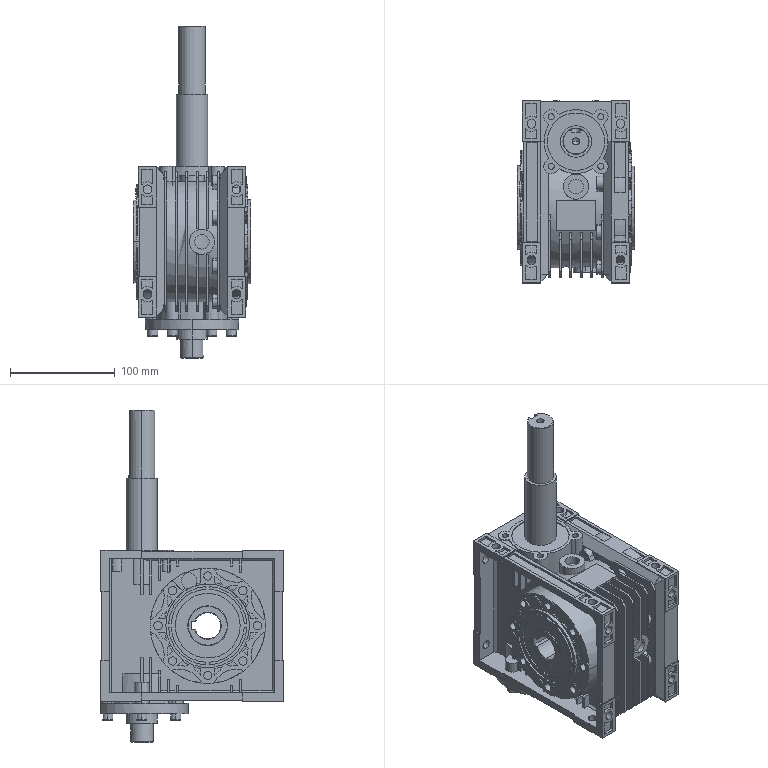Part | SolidWorks | features BaseBody 1 | 1 solid | 1734 faces | box 112 x 174 x 317 mm | volume 1817597 mm3 | plane 991 | cylinder 692 | spline 28 | cone 23 | commonest cylinder face diameters 1 x148 8 x63 13 x38 14.5 x36 14 x34 7 x30